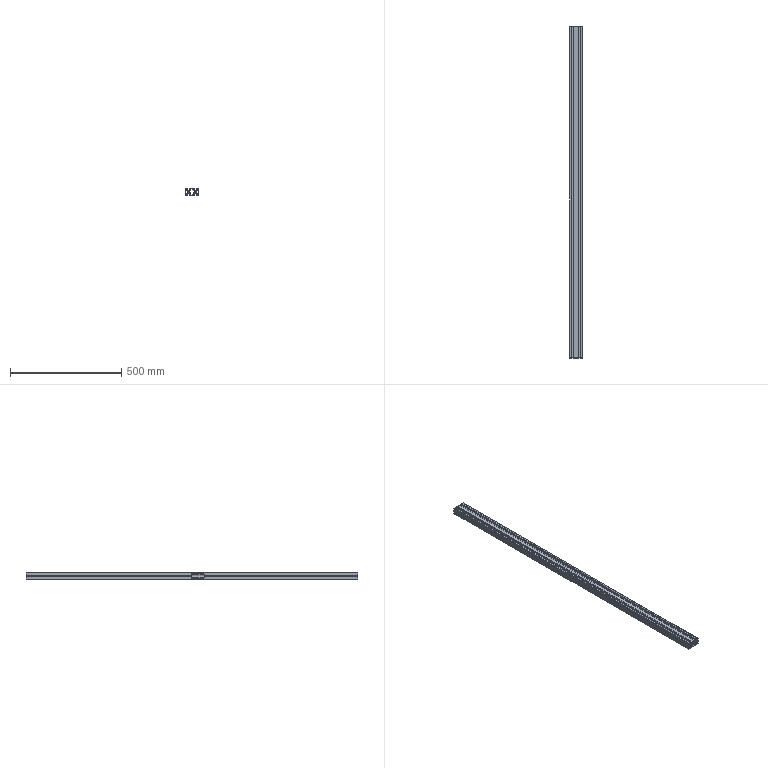Part | STEP file | 02-04 Side frame | 1 solid | 124 faces | box 60 x 1495 x 30 mm | volume 1200559 mm3 | plane 94 | cylinder 30 | commonest cylinder face diameters 6 x8 20.523 x8 2 x6 5 x6 17.044 x2